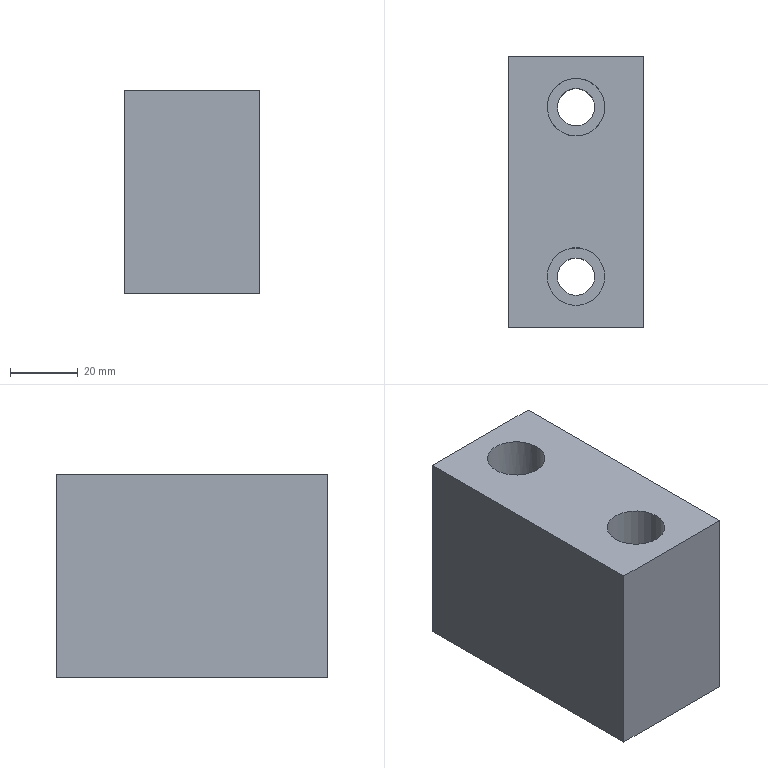Part | NX | features solid 2 | 1 solid | 12 faces | box 40 x 80 x 60 mm | volume 176638 mm3 | plane 8 | cylinder 4 | commonest cylinder face diameters 11 x2 17 x2
STEP:
#1=CARTESIAN_POINT('',(775.,165.,10.));
#2=VERTEX_POINT('',#1);
#3=CARTESIAN_POINT('',(775.,245.,10.));
#4=VERTEX_POINT('',#3);
#5=CARTESIAN_POINT('',(775.,270.,10.));
#6=DIRECTION('',(0.,1.,0.));
#7=VECTOR('',#6,1000.);
#8=LINE('',#5,#7);
#9=EDGE_CURVE('',#2,#4,#8,.T.);
#10=ORIENTED_EDGE('',*,*,#9,.F.);
#11=CARTESIAN_POINT('',(775.,165.,70.));
#12=VERTEX_POINT('',#11);
#13=CARTESIAN_POINT('',(775.,165.,70.));
#14=DIRECTION('',(0.,0.,-1.));
#15=VECTOR('',#14,1000.);
#16=LINE('',#13,#15);
#17=EDGE_CURVE('',#12,#2,#16,.T.);
#18=ORIENTED_EDGE('',*,*,#17,.F.);
#19=CARTESIAN_POINT('',(775.,245.,70.));
#20=VERTEX_POINT('',#19);
#21=CARTESIAN_POINT('',(775.,270.,70.));
#22=DIRECTION('',(0.,1.,0.));
#23=VECTOR('',#22,1000.);
#24=LINE('',#21,#23);
#25=EDGE_CURVE('',#12,#20,#24,.T.);
#26=ORIENTED_EDGE('',*,*,#25,.T.);
#27=CARTESIAN_POINT('',(775.,245.,70.));
#28=DIRECTION('',(0.,0.,-1.));
#29=VECTOR('',#28,1000.);
#30=LINE('',#27,#29);
#31=EDGE_CURVE('',#20,#4,#30,.T.);
#32=ORIENTED_EDGE('',*,*,#31,.T.);
#33=EDGE_LOOP('',(#10,#18,#26,#32));
#34=FACE_BOUND('',#33,.T.);
#35=CARTESIAN_POINT('',(775.,-12.75,70.));
#36=DIRECTION('',(1.,0.,0.));
#37=DIRECTION('',(0.,-1.,0.));
#38=AXIS2_PLACEMENT_3D('',#35,#36,#37);
#39=PLANE('',#38);
#40=ADVANCED_FACE('',(#34),#39,.F.);
#41=CARTESIAN_POINT('',(815.,245.,10.));
#42=VERTEX_POINT('',#41);
#43=CARTESIAN_POINT('',(780.,245.,10.));
#44=DIRECTION('',(1.,0.,0.));
#45=VECTOR('',#44,1000.);
#46=LINE('',#43,#45);
#47=EDGE_CURVE('',#4,#42,#46,.T.);
#48=ORIENTED_EDGE('',*,*,#47,.F.);
#49=ORIENTED_EDGE('',*,*,#31,.F.);
#50=CARTESIAN_POINT('',(815.,245.,70.));
#51=VERTEX_POINT('',#50);
#52=CARTESIAN_POINT('',(780.,245.,70.));
#53=DIRECTION('',(1.,0.,0.));
#54=VECTOR('',#53,1000.);
#55=LINE('',#52,#54);
#56=EDGE_CURVE('',#20,#51,#55,.T.);
#57=ORIENTED_EDGE('',*,*,#56,.T.);
#58=CARTESIAN_POINT('',(815.,245.,70.));
#59=DIRECTION('',(0.,0.,-1.));
#60=VECTOR('',#59,1000.);
#61=LINE('',#58,#60);
#62=EDGE_CURVE('',#51,#42,#61,.T.);
#63=ORIENTED_EDGE('',*,*,#62,.T.);
#64=EDGE_LOOP('',(#48,#49,#57,#63));
#65=FACE_BOUND('',#64,.T.);
#66=CARTESIAN_POINT('',(780.,245.,70.));
#67=DIRECTION('',(0.,-1.,0.));
#68=DIRECTION('',(0.,0.,-1.));
#69=AXIS2_PLACEMENT_3D('',#66,#67,#68);
#70=PLANE('',#69);
#71=ADVANCED_FACE('',(#65),#70,.F.);
#72=CARTESIAN_POINT('',(815.,165.,10.));
#73=VERTEX_POINT('',#72);
#74=CARTESIAN_POINT('',(815.,270.,10.));
#75=DIRECTION('',(0.,-1.,0.));
#76=VECTOR('',#75,1000.);
#77=LINE('',#74,#76);
#78=EDGE_CURVE('',#42,#73,#77,.T.);
#79=ORIENTED_EDGE('',*,*,#78,.F.);
#80=ORIENTED_EDGE('',*,*,#62,.F.);
#81=CARTESIAN_POINT('',(815.,165.,70.));
#82=VERTEX_POINT('',#81);
#83=CARTESIAN_POINT('',(815.,270.,70.));
#84=DIRECTION('',(0.,-1.,0.));
#85=VECTOR('',#84,1000.);
#86=LINE('',#83,#85);
#87=EDGE_CURVE('',#51,#82,#86,.T.);
#88=ORIENTED_EDGE('',*,*,#87,.T.);
#89=CARTESIAN_POINT('',(815.,165.,70.));
#90=DIRECTION('',(0.,0.,-1.));
#91=VECTOR('',#90,1000.);
#92=LINE('',#89,#91);
#93=EDGE_CURVE('',#82,#73,#92,.T.);
#94=ORIENTED_EDGE('',*,*,#93,.T.);
#95=EDGE_LOOP('',(#79,#80,#88,#94));
#96=FACE_BOUND('',#95,.T.);
#97=CARTESIAN_POINT('',(815.,270.,70.));
#98=DIRECTION('',(-1.,0.,0.));
#99=DIRECTION('',(0.,0.,-1.));
#100=AXIS2_PLACEMENT_3D('',#97,#98,#99);
#101=PLANE('',#100);
#102=ADVANCED_FACE('',(#96),#101,.F.);
#103=CARTESIAN_POINT('',(780.,165.,10.));
#104=DIRECTION('',(-1.,0.,0.));
#105=VECTOR('',#104,1000.);
#106=LINE('',#103,#105);
#107=EDGE_CURVE('',#73,#2,#106,.T.);
#108=ORIENTED_EDGE('',*,*,#107,.F.);
#109=ORIENTED_EDGE('',*,*,#93,.F.);
#110=CARTESIAN_POINT('',(780.,165.,70.));
#111=DIRECTION('',(-1.,0.,0.));
#112=VECTOR('',#111,1000.);
#113=LINE('',#110,#112);
#114=EDGE_CURVE('',#82,#12,#113,.T.);
#115=ORIENTED_EDGE('',*,*,#114,.T.);
#116=ORIENTED_EDGE('',*,*,#17,.T.);
#117=EDGE_LOOP('',(#108,#109,#115,#116));
#118=FACE_BOUND('',#117,.T.);
#119=CARTESIAN_POINT('',(780.,165.,70.));
#120=DIRECTION('',(0.,1.,0.));
#121=DIRECTION('',(0.,0.,1.));
#122=AXIS2_PLACEMENT_3D('',#119,#120,#121);
#123=PLANE('',#122);
#124=ADVANCED_FACE('',(#118),#123,.F.);
#125=CARTESIAN_POINT('',(803.5,180.,70.));
#126=VERTEX_POINT('',#125);
#127=CARTESIAN_POINT('',(795.,180.,70.));
#128=DIRECTION('',(0.,0.,1.));
#129=DIRECTION('',(1.,0.,0.));
#130=AXIS2_PLACEMENT_3D('',#127,#128,#129);
#131=CIRCLE('',#130,8.5);
#132=EDGE_CURVE('',#126,#126,#131,.T.);
#133=ORIENTED_EDGE('',*,*,#132,.F.);
#134=EDGE_LOOP('',(#133));
#135=FACE_BOUND('',#134,.T.);
#136=CARTESIAN_POINT('',(803.5,230.,70.));
#137=VERTEX_POINT('',#136);
#138=CARTESIAN_POINT('',(795.,230.,70.));
#139=DIRECTION('',(0.,0.,1.));
#140=DIRECTION('',(1.,0.,0.));
#141=AXIS2_PLACEMENT_3D('',#138,#139,#140);
#142=CIRCLE('',#141,8.5);
#143=EDGE_CURVE('',#137,#137,#142,.T.);
#144=ORIENTED_EDGE('',*,*,#143,.F.);
#145=EDGE_LOOP('',(#144));
#146=FACE_BOUND('',#145,.T.);
#147=ORIENTED_EDGE('',*,*,#25,.F.);
#148=ORIENTED_EDGE('',*,*,#114,.F.);
#149=ORIENTED_EDGE('',*,*,#87,.F.);
#150=ORIENTED_EDGE('',*,*,#56,.F.);
#151=EDGE_LOOP('',(#147,#148,#149,#150));
#152=FACE_BOUND('',#151,.T.);
#153=CARTESIAN_POINT('',(780.,270.,70.));
#154=DIRECTION('',(0.,0.,-1.));
#155=DIRECTION('',(1.,0.,0.));
#156=AXIS2_PLACEMENT_3D('',#153,#154,#155);
#157=PLANE('',#156);
#158=ADVANCED_FACE('',(#135,#146,#152),#157,.F.);
#159=CARTESIAN_POINT('',(800.5,180.,10.));
#160=VERTEX_POINT('',#159);
#161=CARTESIAN_POINT('',(795.,180.,10.));
#162=DIRECTION('',(0.,0.,1.));
#163=DIRECTION('',(1.,0.,0.));
#164=AXIS2_PLACEMENT_3D('',#161,#162,#163);
#165=CIRCLE('',#164,5.5);
#166=EDGE_CURVE('',#160,#160,#165,.T.);
#167=ORIENTED_EDGE('',*,*,#166,.T.);
#168=EDGE_LOOP('',(#167));
#169=FACE_BOUND('',#168,.T.);
#170=CARTESIAN_POINT('',(800.5,230.,10.));
#171=VERTEX_POINT('',#170);
#172=CARTESIAN_POINT('',(795.,230.,10.));
#173=DIRECTION('',(0.,0.,1.));
#174=DIRECTION('',(1.,0.,0.));
#175=AXIS2_PLACEMENT_3D('',#172,#173,#174);
#176=CIRCLE('',#175,5.5);
#177=EDGE_CURVE('',#171,#171,#176,.T.);
#178=ORIENTED_EDGE('',*,*,#177,.T.);
#179=EDGE_LOOP('',(#178));
#180=FACE_BOUND('',#179,.T.);
#181=ORIENTED_EDGE('',*,*,#9,.T.);
#182=ORIENTED_EDGE('',*,*,#47,.T.);
#183=ORIENTED_EDGE('',*,*,#78,.T.);
#184=ORIENTED_EDGE('',*,*,#107,.T.);
#185=EDGE_LOOP('',(#181,#182,#183,#184));
#186=FACE_BOUND('',#185,.T.);
#187=CARTESIAN_POINT('',(780.,270.,10.));
#188=DIRECTION('',(0.,0.,-1.));
#189=DIRECTION('',(1.,0.,0.));
#190=AXIS2_PLACEMENT_3D('',#187,#188,#189);
#191=PLANE('',#190);
#192=ADVANCED_FACE('',(#169,#180,#186),#191,.T.);
#193=CARTESIAN_POINT('',(795.,221.5,55.));
#194=VERTEX_POINT('',#193);
#195=CARTESIAN_POINT('',(795.,230.,55.));
#196=DIRECTION('',(0.,0.,-1.));
#197=DIRECTION('',(0.,-1.,0.));
#198=AXIS2_PLACEMENT_3D('',#195,#196,#197);
#199=CIRCLE('',#198,8.5);
#200=EDGE_CURVE('',#194,#194,#199,.T.);
#201=ORIENTED_EDGE('',*,*,#200,.T.);
#202=EDGE_LOOP('',(#201));
#203=FACE_BOUND('',#202,.T.);
#204=ORIENTED_EDGE('',*,*,#143,.T.);
#205=EDGE_LOOP('',(#204));
#206=FACE_BOUND('',#205,.T.);
#207=CARTESIAN_POINT('',(795.,230.,55.));
#208=DIRECTION('',(0.,0.,1.));
#209=DIRECTION('',(0.,-1.,0.));
#210=AXIS2_PLACEMENT_3D('',#207,#208,#209);
#211=CYLINDRICAL_SURFACE('',#210,8.5);
#212=ADVANCED_FACE('',(#203,#206),#211,.F.);
#213=ORIENTED_EDGE('',*,*,#177,.F.);
#214=EDGE_LOOP('',(#213));
#215=FACE_BOUND('',#214,.T.);
#216=CARTESIAN_POINT('',(795.,235.5,55.));
#217=VERTEX_POINT('',#216);
#218=CARTESIAN_POINT('',(795.,230.,55.));
#219=DIRECTION('',(0.,0.,1.));
#220=DIRECTION('',(0.,1.,0.));
#221=AXIS2_PLACEMENT_3D('',#218,#219,#220);
#222=CIRCLE('',#221,5.5);
#223=EDGE_CURVE('',#217,#217,#222,.F.);
#224=ORIENTED_EDGE('',*,*,#223,.F.);
#225=EDGE_LOOP('',(#224));
#226=FACE_BOUND('',#225,.T.);
#227=CARTESIAN_POINT('',(795.,230.,-35.));
#228=DIRECTION('',(0.,0.,1.));
#229=DIRECTION('',(0.,-1.,0.));
#230=AXIS2_PLACEMENT_3D('',#227,#228,#229);
#231=CYLINDRICAL_SURFACE('',#230,5.5);
#232=ADVANCED_FACE('',(#215,#226),#231,.F.);
#233=ORIENTED_EDGE('',*,*,#223,.T.);
#234=EDGE_LOOP('',(#233));
#235=FACE_BOUND('',#234,.T.);
#236=ORIENTED_EDGE('',*,*,#200,.F.);
#237=EDGE_LOOP('',(#236));
#238=FACE_BOUND('',#237,.T.);
#239=CARTESIAN_POINT('',(795.,230.,55.));
#240=DIRECTION('',(0.,0.,-1.));
#241=DIRECTION('',(0.,1.,0.));
#242=AXIS2_PLACEMENT_3D('',#239,#240,#241);
#243=PLANE('',#242);
#244=ADVANCED_FACE('',(#235,#238),#243,.F.);
#245=CARTESIAN_POINT('',(786.5,180.,55.));
#246=VERTEX_POINT('',#245);
#247=CARTESIAN_POINT('',(795.,180.,55.));
#248=DIRECTION('',(0.,0.,-1.));
#249=DIRECTION('',(-1.,0.,0.));
#250=AXIS2_PLACEMENT_3D('',#247,#248,#249);
#251=CIRCLE('',#250,8.5);
#252=EDGE_CURVE('',#246,#246,#251,.T.);
#253=ORIENTED_EDGE('',*,*,#252,.T.);
#254=EDGE_LOOP('',(#253));
#255=FACE_BOUND('',#254,.T.);
#256=ORIENTED_EDGE('',*,*,#132,.T.);
#257=EDGE_LOOP('',(#256));
#258=FACE_BOUND('',#257,.T.);
#259=CARTESIAN_POINT('',(795.,180.,55.));
#260=DIRECTION('',(0.,0.,1.));
#261=DIRECTION('',(-1.,0.,0.));
#262=AXIS2_PLACEMENT_3D('',#259,#260,#261);
#263=CYLINDRICAL_SURFACE('',#262,8.5);
#264=ADVANCED_FACE('',(#255,#258),#263,.F.);
#265=ORIENTED_EDGE('',*,*,#166,.F.);
#266=EDGE_LOOP('',(#265));
#267=FACE_BOUND('',#266,.T.);
#268=CARTESIAN_POINT('',(800.5,180.,55.));
#269=VERTEX_POINT('',#268);
#270=CARTESIAN_POINT('',(795.,180.,55.));
#271=DIRECTION('',(0.,0.,1.));
#272=DIRECTION('',(1.,0.,0.));
#273=AXIS2_PLACEMENT_3D('',#270,#271,#272);
#274=CIRCLE('',#273,5.5);
#275=EDGE_CURVE('',#269,#269,#274,.F.);
#276=ORIENTED_EDGE('',*,*,#275,.F.);
#277=EDGE_LOOP('',(#276));
#278=FACE_BOUND('',#277,.T.);
#279=CARTESIAN_POINT('',(795.,180.,-35.));
#280=DIRECTION('',(0.,0.,1.));
#281=DIRECTION('',(-1.,0.,0.));
#282=AXIS2_PLACEMENT_3D('',#279,#280,#281);
#283=CYLINDRICAL_SURFACE('',#282,5.5);
#284=ADVANCED_FACE('',(#267,#278),#283,.F.);
#285=ORIENTED_EDGE('',*,*,#275,.T.);
#286=EDGE_LOOP('',(#285));
#287=FACE_BOUND('',#286,.T.);
#288=ORIENTED_EDGE('',*,*,#252,.F.);
#289=EDGE_LOOP('',(#288));
#290=FACE_BOUND('',#289,.T.);
#291=CARTESIAN_POINT('',(795.,180.,55.));
#292=DIRECTION('',(0.,0.,-1.));
#293=DIRECTION('',(1.,0.,0.));
#294=AXIS2_PLACEMENT_3D('',#291,#292,#293);
#295=PLANE('',#294);
#296=ADVANCED_FACE('',(#287,#290),#295,.F.);
#297=CLOSED_SHELL('',(#40,#71,#102,#124,#158,#192,#212,#232,#244,#264,#284,#296));
#298=MANIFOLD_SOLID_BREP('',#297);
#299=(LENGTH_UNIT()NAMED_UNIT(*)SI_UNIT(.MILLI.,.METRE.));
#300=UNCERTAINTY_MEASURE_WITH_UNIT(LENGTH_MEASURE(0.00001),#299,'','');
#301=(NAMED_UNIT(*)PLANE_ANGLE_UNIT()SI_UNIT($,.RADIAN.));
#302=(NAMED_UNIT(*)SI_UNIT($,.STERADIAN.)SOLID_ANGLE_UNIT());
#303=(GEOMETRIC_REPRESENTATION_CONTEXT(3)GLOBAL_UNCERTAINTY_ASSIGNED_CONTEXT((#300))GLOBAL_UNIT_ASSIGNED_CONTEXT((#299,#301,#302))REPRESENTATION_CONTEXT('',''));
#304=ADVANCED_BREP_SHAPE_REPRESENTATION('',(#298),#303);